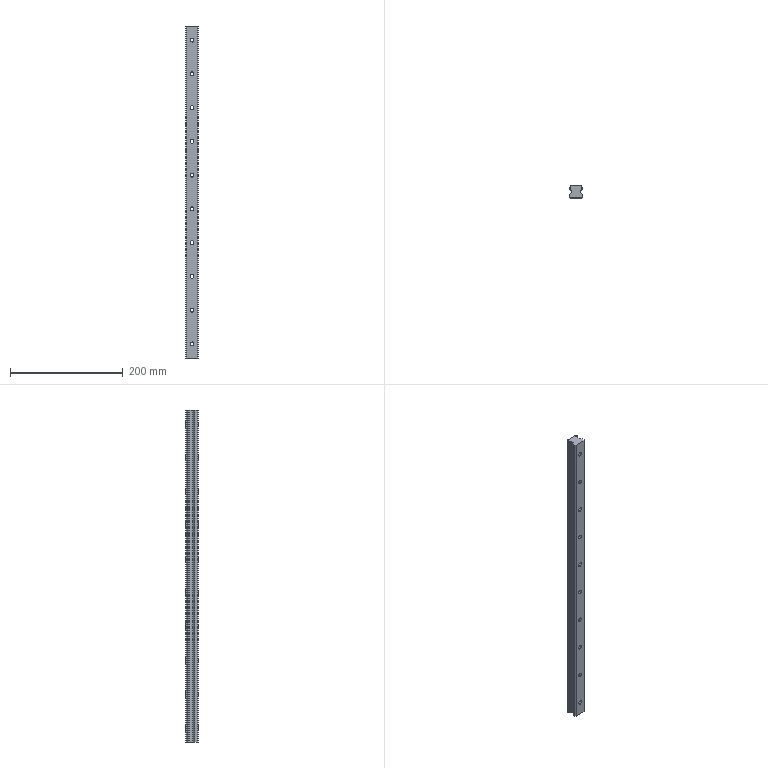Part | SolidWorks | features ICE 2, BaseBody 1, LPattern 1 | 1 solid | 78 faces | box 23 x 22 x 590 mm | volume 242690 mm3 | cylinder 46 | plane 32 | commonest cylinder face diameters 7 x20 11 x20 3.5 x6